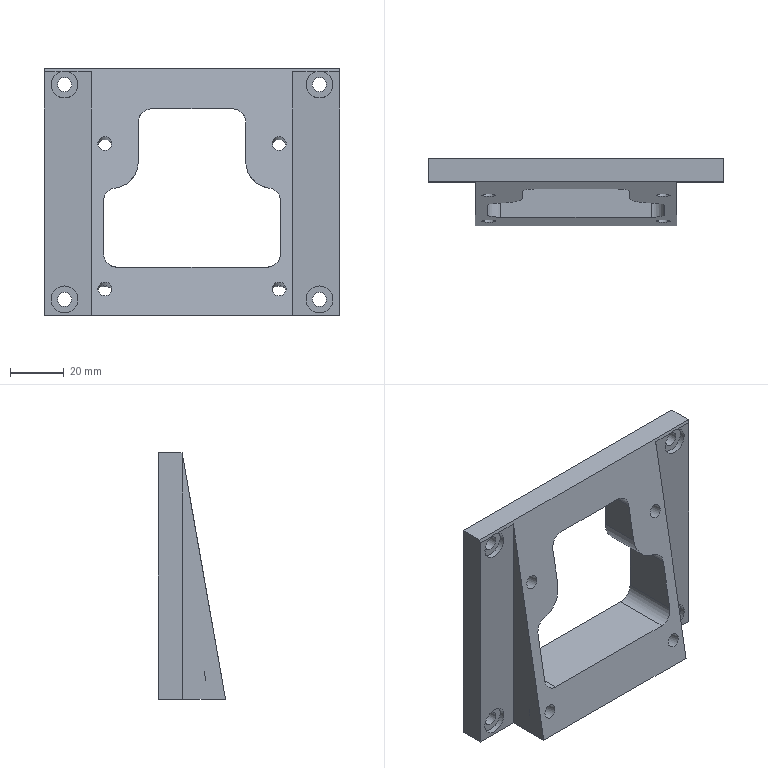CAM job | NX | 3+2 milling, drilling | part box 110 x 25 x 92 mm | stock box 115 x 30 x 100 mm
Tools:
number,name,description,diameter,corner_radius,flute_length,length,flutes
6,D6,平底铣刀-粗,6.0,0.0,25.0,75.0,2
9,D10,平底铣刀-粗,10.0,0.0,35.0,75.0,2
7,D6-J,平底铣刀-精,6.0,0.0,25.0,75.0,2
10,D10-J,平底铣刀-精,10.0,0.0,35.0,75.0,2
1,D80R0.8飞刀,圆鼻刀-粗,80.0,0.8,50.0,75.0,2
17,D6R0.5-J,圆鼻刀-精,6.0,0.5,50.0,75.0,2
2,D6倒角刀,倒角刀,6.0,0.0,3.0,25.0,2
17,ZT5.2,钻头,5.2,0.0,35.0,50.0,2
17,ZT5.3,钻头,5.3,0.0,35.0,50.0,2
Operations:
program,operation,operation_type,tool,method,geometry_group,spindle_rpm,surface_speed,feed_per_tooth,feed_cut,feed_plunge,cut_length_mm,path_length_mm,cut_time_min,machine_time_min
C,底壁铣螺旋开粗-中_COPY_1,VolumeBased25DMillingOperation,D6,分层开粗-切深K-步距G,W-C,8000.0,150.796,0.0938,1500.0,100.0,2374.288,3035.188,1.583,1.649
C,底壁铣螺旋精光-中_COPY_1,VolumeBased25DMillingOperation,D6-J,螺旋精光-切深K-步距G,W-C,8000.0,150.792,0.0625,1000.0,100.0,255.182,921.37,0.2552,0.3218
C,打点-深0.8,Operation,D6倒角刀,NONE,W-C,8000.0,150.796,0.0312,500.0,90.0,7.2,329.666,0.0144,0.0466
C,通孔-5-6,Operation,ZT5.2,NONE,W-C,2800.0,45.742,0.0268,150.0,90.0,42.249,399.764,0.2817,0.3174
B,面铣自动飞面开粗_COPY,FaceMilling,D80R0.8飞刀,分层开粗-切深K-步距G,W-B,4500.0,890.615,0.3333,3000.0,100.0,6044.75,8009.444,2.015,2.211
B,面铣自动飞面精光_COPY,FaceMilling,D80R0.8飞刀,侧刃精光-切深K-步距G,W-B,4500.0,890.615,0.1111,1000.0,100.0,684.0,780.0,0.684,0.6936
B,型腔铣开粗-中_COPY_1,CavityMilling,D10,分层开粗-切深K-步距G,W-B,8000.0,251.32,0.25,4000.0,100.0,47535.923,49015.789,11.884,12.1
B,底壁铣螺旋开粗-中_COPY,VolumeBased25DMillingOperation,D6,分层开粗-切深K-步距G,W-B,8000.0,150.792,0.1875,3000.0,100.0,320.942,1103.478,0.107,0.1852
B,底壁铣螺旋精光-中_COPY,VolumeBased25DMillingOperation,D6-J,螺旋精光-切深K-步距G,W-B,8000.0,150.792,0.0625,1000.0,100.0,145.692,933.573,0.1457,0.2245
B,等高精光往复爬面_COPY,ZLevelMilling,D6R0.5-J,等高爬面-切深K-步距G,W-B,9000.0,169.646,0.25,4500.0,100.0,45003.792,45159.453,10.001,10.016
B,平面去毛刺6X45L_COPY,SurfaceContour,D6倒角刀,爬面_倒角-切深0-步距G,W-B,6500.0,122.519,0.1154,1500.0,100.0,423.208,1348.062,0.2821,0.3746
B,底壁铣精光底面-中_COPY,VolumeBased25DMillingOperation,D10-J,精光步距切深关,W-B,7000.0,175.0,0.0536,1500.0,100.0,824.514,1064.66,0.5497,0.5737
B,底壁铣精光侧面-中-选底面_COPY,VolumeBased25DMillingOperation,D10-J,侧刃精光-切深K-步距G,W-B,8000.0,251.32,0.0625,1000.0,100.0,218.763,374.815,0.2188,0.2344
B,底壁铣精光侧面-中-选底面_COPY_1,VolumeBased25DMillingOperation,D10-J,侧刃精光-切深K-步距G,W-B,8000.0,251.32,0.0625,1000.0,100.0,218.764,374.809,0.2188,0.2344
A,顶面,FaceMilling,D80R0.8飞刀,侧刃精光-切深K-步距G,W-A,4500.0,1385.0,0.1667,1500.0,100.0,670.0,766.0,0.4467,0.4563
A,外形粗_2,VolumeBased25DMillingOperation,D10,METHOD,W-A,8000.0,251.327,0.375,6000.0,80.0,14390.983,14514.483,2.398,2.411
A,型腔铣开粗-中_COPY,CavityMilling,D10,分层开粗-切深K-步距G,W-A,8000.0,251.32,0.25,4000.0,100.0,26151.629,27103.124,6.538,6.68
A,打点,Operation,D6倒角刀,METHOD,W-A,8000.0,150.796,0.1562,2500.0,0.0,10.0,378.018,0.004,0.0408
A,打孔,Operation,ZT5.3,METHOD,W-A,3000.0,49.951,0.2,1200.0,0.0,52.0,462.018,0.0433,0.0843
A,框半精_1,VolumeBased25DMillingOperation,D6-J,METHOD,W-A,8000.0,100.531,0.0625,1000.0,100.0,1078.937,1226.433,1.079,1.094
A,仅选体,SurfaceContour,D6倒角刀,METHOD,W-A,8000.0,150.796,0.1875,3000.0,100.0,536.976,820.459,0.179,0.2073
A,铣倒角_1,PlanarMilling,D6倒角刀,METHOD,W-A,8000.0,150.796,0.0375,600.0,100.0,42.539,707.94,0.0709,0.1374
A,外形半精_2,VolumeBased25DMillingOperation,D6-J,METHOD,W-A,9000.0,169.646,0.0667,1200.0,100.0,1283.297,1685.338,1.069,1.11